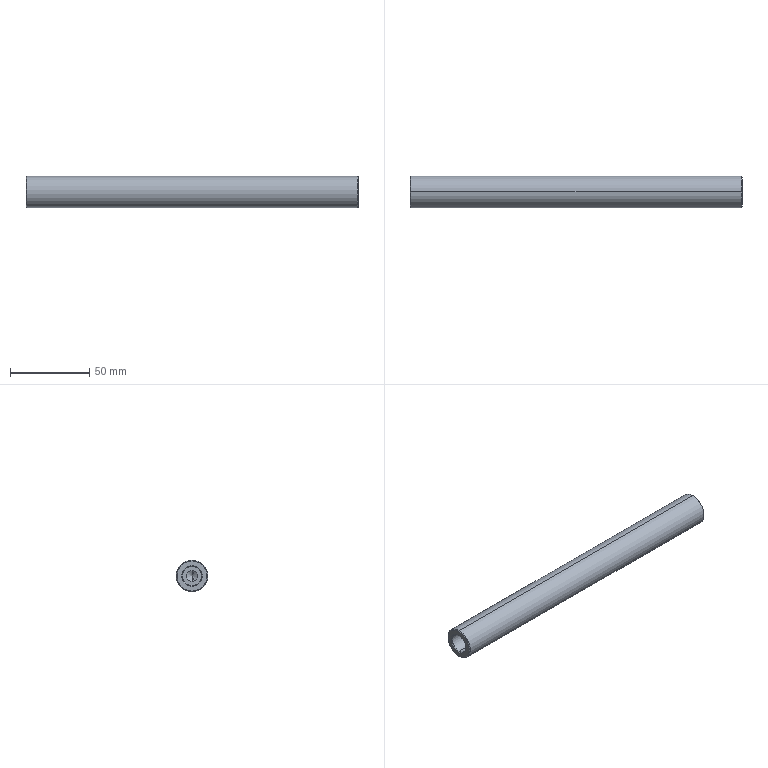Part | STEP file | 0228_204_Shaft | 1 solid | 26 faces | box 210 x 20 x 20 mm | volume 61901 mm3 | cone 12 | cylinder 10 | plane 4 | commonest cylinder face diameters 6.8 x4 12 x4 20 x2